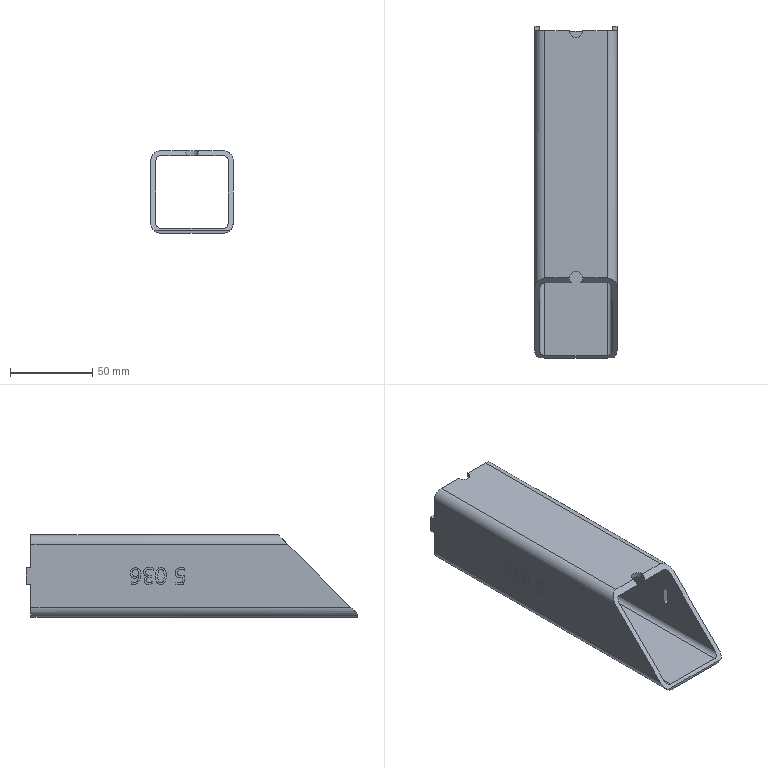Part | SolidWorks | features BaseBody 1 | 1 solid | 95 faces | box 50 x 201.5 x 50 mm | volume 94471 mm3 | plane 44 | spline 39 | cylinder 12 | commonest cylinder face diameters 6 x4 8 x4 12 x4